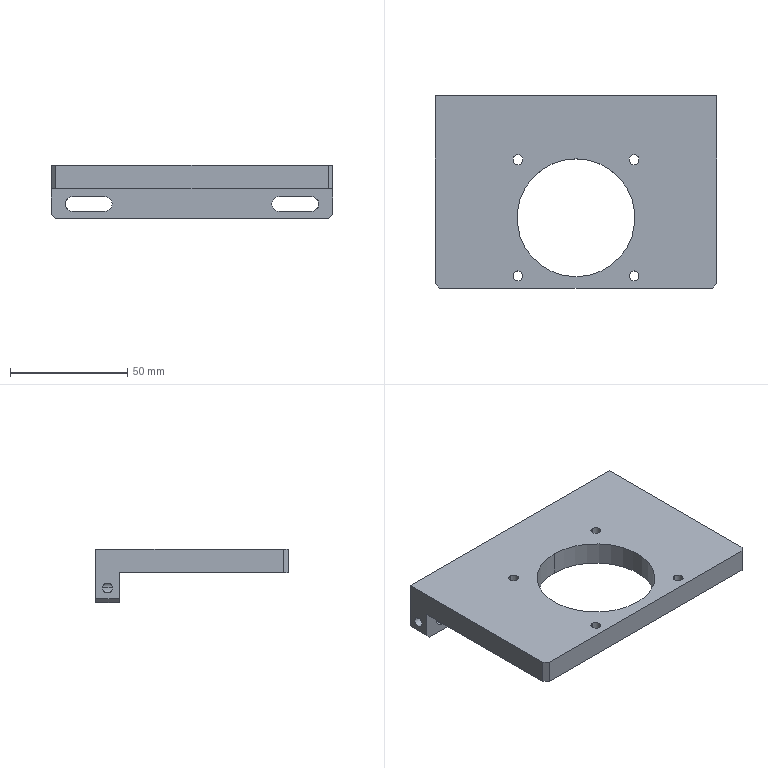NC program | NX | posted with a generic post | part box 120 x 82 x 22.8 mm
Lines 2187 to 2242 of 2242:
(PLANAR_MILL_COPY_COPY_2 , TOOL : D6A45)
N4372 T01 M6
N4374 G54
N4376 G17 G0 G90 X44.866 Y6.85 B0. C0. S9500 M3
N4378 G43 Z30. H1
N4380 Z0.5
N4382 G94 G1 Z-1. F1250.
N4384 G3 X44. Y7.35 R1.
N4386 G1 X37.15
N4388 G3 X34.9 Y5.1 R2.25
N4390 X37.15 Y2.85 R2.25
N4392 G1 X50.85
N4394 G3 X53.1 Y5.1 R2.25
N4396 X50.85 Y7.35 R2.25
N4398 G1 X44.
N4400 G3 X43.134 Y6.85 R1.
N4402 G1 Z0.5
N4404 G0 Z30.
N4406 X0.866 Y-12.8
N4408 Z0.5
N4410 G1 Z-1.
N4412 G3 X0. Y-12.3 R1.
N4414 G1 X-60.
N4416 G2 X-60.9 Y-11.4 R0.9
N4418 G1 Y9.6
N4420 G2 X-60.636 Y10.236 R0.9
N4422 G1 X-58.836 Y12.036
N4424 G2 X-58.2 Y12.3 R0.9
N4426 G1 X58.2
N4428 G2 X58.836 Y12.036 R0.9
N4430 G1 X60.636 Y10.236
N4432 G2 X60.9 Y9.6 R0.9
N4434 G1 Y-11.4
N4436 G2 X60. Y-12.3 R0.9
N4438 G1 X0.
N4440 G3 X-0.866 Y-12.8 R1.
N4442 G1 Z0.5
N4444 G0 Z30.
N4446 X-43.134 Y6.85
N4448 Z0.5
N4450 G1 Z-1.
N4452 G3 X-44. Y7.35 R1.
N4454 G1 X-50.85
N4456 G3 X-53.1 Y5.1 R2.25
N4458 X-50.85 Y2.85 R2.25
N4460 G1 X-37.15
N4462 G3 X-34.9 Y5.1 R2.25
N4464 X-37.15 Y7.35 R2.25
N4466 G1 X-44.
N4468 G3 X-44.866 Y6.85 R1.
N4470 G1 Z0.5
N4472 G0 Z30.
N4474 M5
N4476 M2